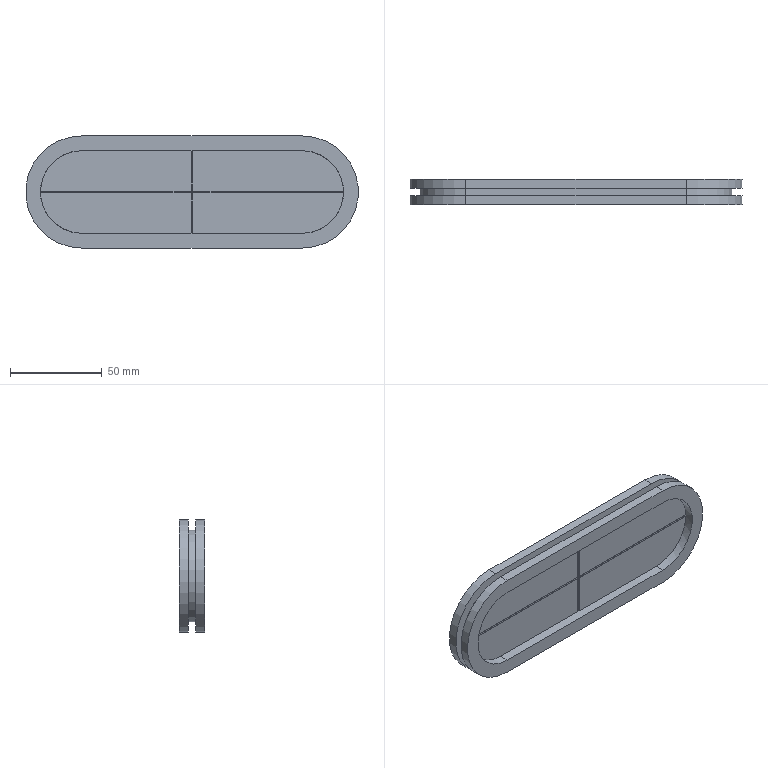Part | SolidWorks | features BaseBody 1 | 1 solid | 54 faces | box 181 x 14 x 61 mm | volume 64291 mm3 | plane 44 | cylinder 10 | commonest cylinder face diameters 45 x4 61 x4 50 x2